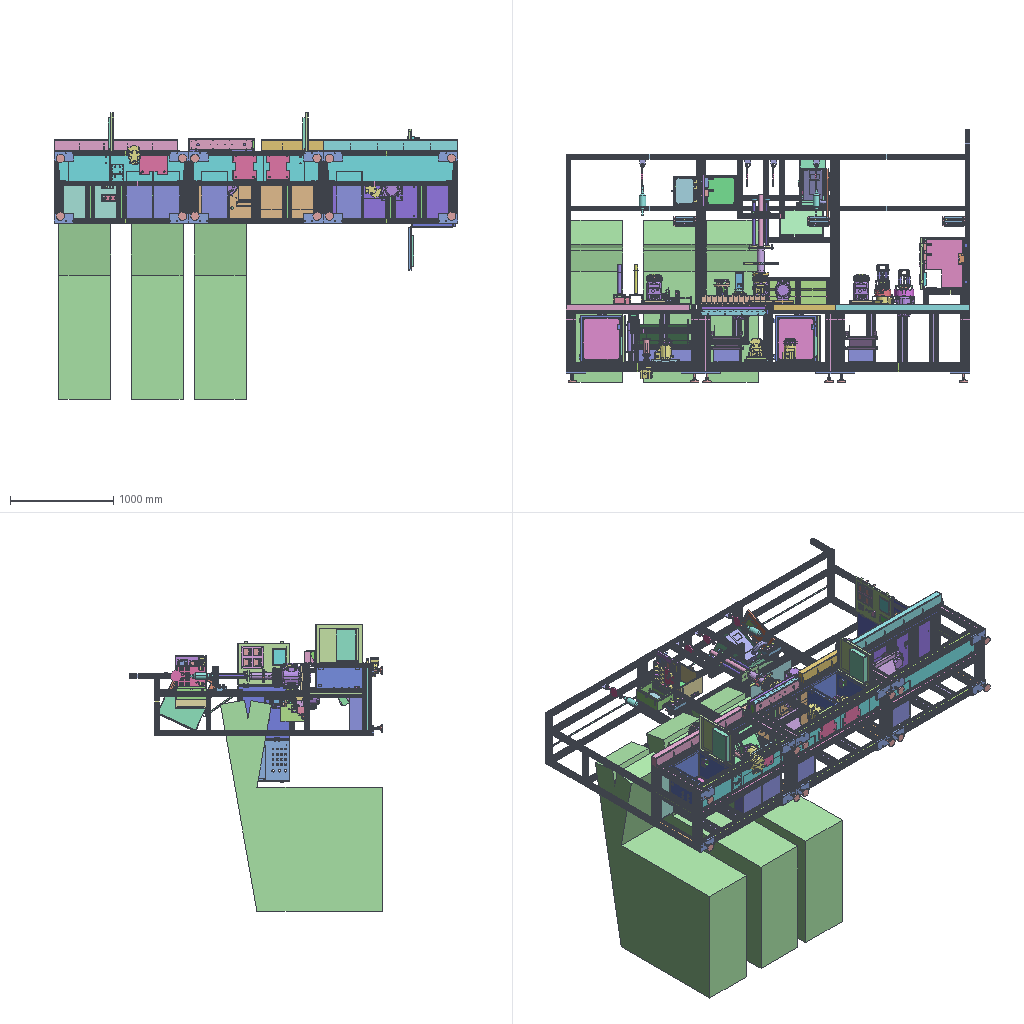Assembly | STEP file | 253 different items | 762 placed | box 3900 x 2440 x 2771 mm
Parts list (item | name | quantity | parent item | size | volume):
1 | Foot pad | x12 | in 1300 standard stand 3 | 80 x 145 x 80 mm | 114495 mm3
2 | Foot seat plate 2 | x12 | in 1300 standard stand 3 | 190 x 100 x 20 mm | 368452 mm3
3 | 4590-1120 aluminium profile (bottom rear cross 2) | x6 | in 1300 standard stand 3 | 90 x 45 x 1120 mm | 1313429 mm3
4 | 4590-705 Al 3 (front col) | x6 | in 1300 standard stand 3 | 90 x 45 x 558 mm | 654369 mm3
5 | 4590-600 Al (base long) | x6 | in 1300 standard stand 3 | 90 x 45 x 610 mm | 715349 mm3
6 | 4590-705 aluminium profile (rear column 2) | x6 | in 1300 standard stand 3 | 90 x 45 x 603 mm | 707141 mm3
7 | 4590-615 aluminium profile (rear middle upright 2) | x9 | in 1300 standard stand 3 | 90 x 45 x 513 mm | 601597 mm3
8 | 4590 aluminium profile (middle longitudinal 3) | x15 | in 1300 standard stand 3 | 90 x 45 x 700 mm | 820893 mm3
9 | 4545-1210 aluminium profile (upper long) | x12 | in 1300 standard stand 3 | 45 x 45 x 1407 mm | 976243 mm3
10 | 4545-1210 aluminium profile (upper cross long) | x14 | in 1300 standard stand 3 | 45 x 45 x 1210 mm | 839555 mm3
11 | 4545-765 aluminium profile (upper short) | x6 | in 1300 standard stand 3 | 45 x 45 x 597.5 mm | 414574 mm3
12 | SOP hanger seat | x6 | in 1300 standard stand 3 | 50 x 30 x 28 mm | 13038 mm3
13 | SOP hanger | x3 | in 1300 standard stand 3 | 12 x 12 x 1210 mm | 136812 mm3
14 | 4545-390 Al (side support) | x6 | in 1300 standard stand 3 | 45 x 45 x 335 mm | 232439 mm3
15 | 4590-1300 | x3 | in 1300 standard stand 3 | 90 x 45 x 1300 mm | 1524515 mm3
16 | 4590 Al (column) | x6 | in 1300 standard stand 3 | 90 x 45 x 513 mm | 601597 mm3
17 | 4590-1210 aluminium profile | x3 | in 1300 standard stand 3 | 90 x 45 x 1210 mm | 1418972 mm3
18 | Jig plate | x3 | in 1300 standard stand 3 | 1300 x 337.75 x 2 mm | 788863 mm3
19 | 10P30 assy jig base | x3 | in 10P30 assy locating jig | 230 x 270 x 25 mm | 1350745 mm3
20 | PN_0001 cylinder body | x7 | in 10P30 | 246.9 x 192 x 142 mm | 3389900 mm3
21 | PN_0001 rotor | x8 | in 10P30, Rotor mis-part check fixture | 43.5 x 155 x 155 mm | 349048 mm3
22 | 10P30 rotor 2 | x8 | in 10P30, Rotor mis-part check fixture | 43.5 x 156.4 x 156.4 mm | 346928 mm3
23 | 10P30 rotor clip | x8 | in 10P30, Circlip fixture (PN_0001 rotor) | 48.3 x 51.304 x 1.75 mm | 1045 mm3
24 | 10P30 hub | x8 | in 10P30, Shim selector hub step measuring fixture | 45 x 134.5 x 134.5 mm | 158986 mm3
25 | 10P30 stator | x7 | in 10P30 | 133.205 x 156.603 x 50 mm | 289241 mm3
26 | prevailing torque hex nuts with flange gb_PreviewCfg | x7 | in 10P30 | 11.8 x 11.8 x 5.3 mm | 298.912 mm3
27 | Fixture base plate | x6 | in 10P30 assy locating jig, Mkt assy locating jig | 270 x 230 x 15 mm | 846944 mm3
28 | Market locating fixture base plate | x3 | in Mkt assy locating jig | 230 x 270 x 25 mm | 1234801 mm3
29 | Market cylinder body | x7 | in Market, Stator circlip shortage check fixture | 195.5 x 183.011 x 125.785 mm | 2010849 mm3
30 | Market rotor | x7 | in Market, Rotor mis-part check fixture | 30.5 x 135 x 135 mm | 165270 mm3
31 | Mkt rotor clip | x7 | in Market, Circlip fixture (market rotor) | 41.6 x 41.383 x 1 mm | 557.011 mm3
32 | Market stator | x6 | in Market | 29.5 x 96.5 x 96.5 mm | 131288 mm3
33 | Mkt stator clip | x9 | in Market, Stator circlip shortage check fixture, Circlip fixture (market stator) | 43.8 x 47.287 x 1.8 mm | 874.267 mm3
34 | Mkt hub | x7 | in Market, Shim selector hub step measuring fixture | 38 x 105 x 105 mm | 81740 mm3
35 | hexagon flange bolts--small series gb_PreviewCfg | x6 | in Market | 31.8 x 13.6 x 13.6 mm | 1212 mm3
36 | Outer collar ring | x1 | in Stator circlip shortage check fixture | 72 x 72 x 57 mm | 42154 mm3
37 | Inner collar ring | x1 | in Stator circlip shortage check fixture | 41 x 41 x 43 mm | 18386 mm3
38 | Sensing post | x1 | in Stator circlip shortage check fixture | 11 x 15 x 29 mm | 1328 mm3
39 | Sensor mounting seat | x1 | in Stator circlip shortage check fixture | 72 x 72 x 46.3 mm | 26633 mm3
40 | Fix sleeve | x1 | in Stator circlip shortage check fixture | 72 x 72 x 150.6 mm | 87626 mm3
41 | Sensor nut | x1 | in Stator circlip shortage check fixture | 13 x 13.856 x 16.3 mm | 789.56 mm3
42 | Sensor head GT2-H12 | x1 | in Stator circlip shortage check fixture | 28 x 118.4 x 16 mm | 29940 mm3
43 | Return spring | x1 | in Stator circlip shortage check fixture | 32.75 x 32.75 x 12.75 mm | 176.657 mm3
44 | Stator clip std part | x1 | in Stator circlip shortage check fixture | 22 x 70 x 70 mm | 50341 mm3
45 | Stator circlip gauge hook | x1 | in Stator circlip shortage check fixture | 70 x 102 x 6 mm | 7420 mm3
46 | Spring hanging buckle | x4 | in Spring scale hook | 70 x 82.5 x 5 mm | 17833 mm3
47 | Spring hanger hook | x4 | in Spring scale hook | 18 x 8 x 120 mm | 16287 mm3
48 | Spring scale | x4 | in Spring scale hook | 106.116 x 223.189 x 10 mm | 107592 mm3
49 | Base-10P30 rotor clip | x1 | in Circlip fixture (PN_0001 rotor) | 120 x 86 x 10 mm | 99024 mm3
50 | Circlip fixture-upright plate | x8 | in Circlip fixture (PN_0001 rotor), Circlip fixture (market stator), Circlip fixture (market rotor) | 86 x 80 x 10 mm | 66708 mm3
51 | Clip jig-top plate | x4 | in Circlip fixture (PN_0001 rotor), Circlip fixture (market stator), Circlip fixture (market rotor) | 120 x 76 x 10 mm | 73644 mm3
52 | Clip jig-column 1 | x4 | in Circlip fixture (PN_0001 rotor), Circlip fixture (market stator), Circlip fixture (market rotor) | 15 x 12 x 291 mm | 49759 mm3
53 | Conn plate L | x3 | in Circlip fixture (PN_0001 rotor), Circlip fixture (market stator) | 40 x 288.5 x 1 mm | 11349 mm3
54 | Circlip fixture-medium storage post | x1 | in Circlip fixture (PN_0001 rotor) | 39 x 38.994 x 288.5 mm | 253295 mm3
55 | Strip (L) | x3 | in Circlip fixture (PN_0001 rotor), Circlip fixture (market stator) | 15 x 2 x 288.5 mm | 8464 mm3
56 | Photo seat | x8 | in Circlip fixture (PN_0001 rotor), Circlip fixture (market stator), Circlip fixture (market rotor) | 35 x 20 x 2 mm | 1235 mm3
57 | Circlip fixture-column 2 | x4 | in Circlip fixture (PN_0001 rotor), Circlip fixture (market stator), Circlip fixture (market rotor) | 15 x 12 x 291 mm | 51262 mm3
58 | Base plate-market stator circlip | x2 | in Circlip fixture (market stator) | 120 x 86 x 10 mm | 98205 mm3
59 | Circlip fixture-large storage post | x2 | in Circlip fixture (market stator) | 35.5 x 35.493 x 288.5 mm | 209417 mm3
60 | Base plate-market rotor circlip | x1 | in Circlip fixture (market rotor) | 120 x 86 x 10 mm | 97902 mm3
61 | Press strip (small) | x1 | in Circlip fixture (market rotor) | 12 x 2 x 289.5 mm | 6757 mm3
62 | Conn plate (S) | x1 | in Circlip fixture (market rotor) | 35 x 289.5 x 1 mm | 9942 mm3
63 | Clip jig-small post | x1 | in Circlip fixture (market rotor) | 30 x 29.992 x 289.3 mm | 149299 mm3
64 | Rotor mismatch side plate | x2 | in Rotor mis-part check fixture | 200 x 65 x 12 mm | 150424 mm3
65 | Rotor mis-part check fixture-guide rod | x4 | in Rotor mis-part check fixture | 12 x 12 x 210 mm | 23681 mm3
66 | Rotor mis-part check fixture-base plate | x1 | in Rotor mis-part check fixture | 440 x 200 x 11 mm | 944706 mm3
67 | Rotor mismatch mid plate | x2 | in Rotor mis-part check fixture | 200 x 54 x 12 mm | 123822 mm3
68 | Rotor mis-part check fixture-go gauge 1 | x1 | in Rotor mis-part check fixture | 200 x 120 x 12 mm | 206238 mm3
69 | Rotor mismatch gauge 2 | x1 | in Rotor mis-part check fixture | 200 x 120 x 12 mm | 185907 mm3
70 | Rotor mismatch gauge 3 | x1 | in Rotor mis-part check fixture | 200 x 120 x 12 mm | 185482 mm3
71 | Rotor detection photoelectric sensor | x2 | in Rotor mis-part check fixture | 29.674 x 4 x 54.352 mm | 340.68 mm3
72 | Rotor photoelectric sensor bracket | x1 | in Rotor mis-part check fixture | 80 x 106 x 15 mm | 26188 mm3
73 | Proximity mount-rotor | x2 | in Rotor mis-part check fixture | 66 x 40 x 20 mm | 4954 mm3
74 | Knob plunger PMXYK10 | x2 | in Rotor mis-part check fixture | 18 x 52 x 18 mm | 5094 mm3
75 | Guide rod connection | x2 | in Rotor mis-part check fixture | 12 x 11 x 16 mm | 1579 mm3
76 | hexagon socket head cap screws gb_PreviewCfg | x6 | in Rotor mis-part check fixture, 35N wrench lock | 7.6 x 3 x 3 mm | 21.652 mm3
77 | Shim select base | x1 | in Shim selector hub step measuring fixture | 150 x 150 x 12 mm | 250622 mm3
78 | Column | x3 | in Shim selector hub step measuring fixture | 16 x 16 x 160 mm | 30717 mm3
79 | Shim selection fixture body | x1 | in Shim selector hub step measuring fixture | 150 x 150 x 50 mm | 396055 mm3
80 | GS-1713 (Ono) | x11 | in Shim selector hub step measuring fixture, Rotor step measuring fixture-PN_0001, Clearance measuring fixture-PN_0001, Gap jig-Mkt | 18 x 33 x 141.5 mm | 52927 mm3
81 | GS mount plate | x1 | in Shim selector hub step measuring fixture | 50 x 75 x 8 mm | 29332 mm3
82 | Guide post | x1 | in Shim selector hub step measuring fixture | 10 x 12 x 44 mm | 1435 mm3
83 | Spring-hub step test | x1 | in Shim selector hub step measuring fixture | 8.7 x 8.7 x 23.95 mm | 74.991 mm3
84 | Guide post cap | x1 | in Shim selector hub step measuring fixture | 11.5 x 11.5 x 8 mm | 657.251 mm3
85 | PN_0001 hub standard part | x1 | in Shim selector hub step measuring fixture | 134.5 x 134.5 x 16.35 mm | 127475 mm3
86 | Mkt hub std part | x1 | in Shim selector hub step measuring fixture | 105 x 105 x 11.7 mm | 77844 mm3
87 | Prox bracket-hub | x1 | in Shim selector hub step measuring fixture | 56 x 10 x 18 mm | 1998 mm3
88 | Probe guide bush JBA6-16 | x1 | in Shim selector hub step measuring fixture | 10 x 10 x 16 mm | 793.757 mm3
89 | Limit sleeve | x1 | in Shim selector hub step measuring fixture | 18.5 x 20 x 42.5 mm | 8069 mm3
90 | Sensor fixing block-10P30 | x1 | in Rotor step measuring fixture-PN_0001 | 70 x 80 x 57 mm | 133616 mm3
91 | Rotor locating claw-PN_0001 | x1 | in Rotor step measuring fixture-PN_0001 | 91.977 x 95 x 57 mm | 127328 mm3
92 | Small circlip installation check head-PN_0001 | x1 | in Rotor step measuring fixture-PN_0001 | 70 x 70 x 15.85 mm | 18313 mm3
93 | Circlip check locating post-PN_0001 | x3 | in Rotor step measuring fixture-PN_0001 | 15 x 15 x 52.5 mm | 2401 mm3
94 | Sensor mount plate | x10 | in Rotor step measuring fixture-PN_0001, Clearance measuring fixture-PN_0001, Gap jig-Mkt | 15 x 15 x 26 mm | 1338 mm3
95 | Rotor step probe-10P30 | x1 | in Rotor step measuring fixture-PN_0001 | 25 x 25 x 61.5 mm | 22119 mm3
96 | Rotor step cover | x1 | in Rotor step measuring fixture-PN_0001 | 85 x 75 x 160 mm | 109085 mm3
97 | Spring-circlip check | x1 | in Rotor step measuring fixture-PN_0001 | 41.5 x 41.5 x 26.5 mm | 1389 mm3
98 | Spring-rotor test | x1 | in Rotor step measuring fixture-PN_0001 | 18.75 x 18.75 x 28.75 mm | 175.083 mm3
99 | Rotor step bushing JBH8-12 | x3 | in Rotor step measuring fixture-PN_0001 | 16 x 16 x 16 mm | 1313 mm3
100 | hex nuts, style 1-grades ab gb_PreviewCfg | x3 | in Rotor step measuring fixture-PN_0001 | 18.475 x 16 x 8.4 mm | 1302 mm3
101 | Seat bracket-10P30 | x1 | in Rotor step measuring fixture-PN_0001 | 150 x 120 x 50 mm | 90314 mm3
102 | Seat-PN_0001 | x1 | in Rotor step measuring fixture-PN_0001 | 105 x 105 x 30 mm | 196684 mm3
103 | 35N torque tester | x1 | in 35N wrench lock | 54 x 85 x 717 mm | 972742 mm3
104 | Hex head-Mkt | x1 | in 35N wrench lock | 21 x 21 x 80 mm | 24655 mm3
105 | Hub mounting plate | x1 | in 35N wrench lock | 155 x 155 x 30 mm | 252907 mm3
106 | Connecting tube sleeve | x1 | in 35N wrench lock | 70 x 70 x 230 mm | 273867 mm3
107 | Bush plate | x1 | in 35N wrench lock | 180 x 180 x 15 mm | 370713 mm3
108 | Handle seat new 2 | x1 | in 35N wrench lock | 68.5 x 120 x 20 mm | 86648 mm3
109 | Handle seat new 1 | x1 | in 35N wrench lock | 68.5 x 120 x 20 mm | 85047 mm3
110 | Handle new | x2 | in 35N wrench lock | 20 x 20 x 112 mm | 31180 mm3
111 | A2A-4B | x1 | in 35N wrench lock | 20 x 41.8 x 14 mm | 7935 mm3
112 | Wrench hook | x2 | in 35N wrench lock | 26 x 26 x 6 mm | 1260 mm3
113 | Linear bearing LMH25UU | x2 | in 35N wrench lock | 59 x 62 x 46 mm | 53686 mm3
114 | 25 guide rod | x2 | in 35N wrench lock | 25 x 25 x 450 mm | 219459 mm3
115 | Wrench mounting plate | x1 | in 35N wrench lock | 240 x 100 x 15 mm | 319377 mm3
116 | 4545 profile 1 | x2 | in 35N wrench lock | 45 x 45 x 450 mm | 312231 mm3
117 | Hard stop block | x2 | in 35N wrench lock | 50 x 50 x 20 mm | 36960 mm3
118 | Buffer sleeve | x2 | in 35N wrench lock | 50 x 50 x 20 mm | 26853 mm3
119 | 4545 profile 2 | x2 | in 35N wrench lock | 45 x 45 x 535 mm | 371208 mm3
120 | 4545 profile 3 | x2 | in 35N wrench lock | 45 x 45 x 90 mm | 62446 mm3
121 | Hub chuck-Mkt | x1 | in 35N wrench lock | 135 x 135 x 18 mm | 146789 mm3
122 | Hex head-PN_0001 | x1 | in 35N wrench lock | 21 x 21 x 90 mm | 27340 mm3
123 | Hub chuck-10P | x1 | in 35N wrench lock | 135 x 135 x 18 mm | 101128 mm3
124 | Torsion pin | x2 | in 35N wrench lock | 10 x 10 x 20 mm | 1542 mm3
125 | Torque wrench | x2 | - | 63.096 x 292.35 x 63.096 mm | 430044 mm3
126 | Screw lock-base plate PN_0001 | x1 | in Screw lock jig 10P30 | 270 x 200 x 25 mm | 1267432 mm3
127 | Screw jig plate | x2 | in Screw lock jig 10P30, Screw lock locating fixture-market | 200 x 270 x 15 mm | 725684 mm3
128 | Flange-10P30 | x1 | in Clearance measuring fixture-PN_0001 | 168 x 168 x 42 mm | 255273 mm3
129 | Conductive post-PN_0001 | x1 | in Clearance measuring fixture-PN_0001 | 11 x 11 x 94 mm | 4420 mm3
130 | Handle rod | x2 | in Clearance measuring fixture-PN_0001, Gap jig-Mkt | 32 x 32 x 94 mm | 15016 mm3
131 | Handle seat | x2 | in Clearance measuring fixture-PN_0001, Gap jig-Mkt | 137 x 24.5 x 15 mm | 45015 mm3
132 | Gap jig seat-10P30 | x1 | in Clearance measuring fixture-PN_0001 | 190 x 190 x 65 mm | 588080 mm3
133 | Fixture seat bracket-PN_0001 | x1 | in Clearance measuring fixture-PN_0001 | 200 x 200 x 80 mm | 215628 mm3
134 | Locating post-10P30 | x1 | in Clearance measuring fixture-PN_0001 | 65 x 65 x 33 mm | 42831 mm3
135 | Handle | x2 | in Clearance measuring fixture-PN_0001, Gap jig-Mkt | 137 x 42 x 26 mm | 58032 mm3
136 | Spring | x2 | in Clearance measuring fixture-PN_0001, Gap jig-Mkt | 10.75 x 10.75 x 22 mm | 58.932 mm3
137 | Proximity mounting bent plate | x2 | in Clearance measuring fixture-PN_0001, Gap jig-Mkt | 30 x 32 x 45 mm | 1657 mm3
138 | Guard post | x8 | in Clearance measuring fixture-PN_0001, Gap jig-Mkt | 10 x 10 x 45 mm | 3034 mm3
139 | Station two ctrl box body | x1 | in Station two ctrl box | 310 x 300 x 225.796 mm | 688947 mm3
140 | Station two ctrl box cover | x1 | in Station two ctrl box | 300 x 20 x 300 mm | 151242 mm3
141 | Station two mount plate | x1 | in Station two ctrl box | 270 x 270 x 17 mm | 174541 mm3
142 | Amplifier | x6 | in Station two ctrl box, Station three ctrl box | 72 x 72 x 119 mm | 337581 mm3
143 | Shim selection | x1 | in Station two ctrl box | 96 x 96 x 119 mm | 593520 mm3
144 | Button | x10 | in Station two ctrl box, Station three ctrl box | 24 x 20 x 39 mm | 10735 mm3
145 | Display 1 | x2 | in Station two ctrl box, Station three ctrl box | 68 x 33 x 10 mm | 22440 mm3
146 | Selector switch | x1 | in Station two ctrl box | 25 x 25 x 30 mm | 7576 mm3
147 | DIP switch | x3 | in Station two ctrl box | 40 x 30 x 5.5 mm | 6025 mm3
148 | Hinge leaf | x8 | in Station two ctrl box, Station three ctrl box | 25.5 x 24.5 x 54 mm | 7881 mm3
149 | Hinge shaft | x6 | in Station two ctrl box, Station three ctrl box | 6 x 54 x 6 mm | 1527 mm3
150 | Station two plug plate low | x2 | in Station two ctrl box | 85 x 10 x 17.5 mm | 12524 mm3
151 | Station two plug plate up | x2 | in Station two ctrl box | 85 x 10 x 17.5 mm | 11964 mm3
152 | DIP switch expansion board | x1 | in Station two ctrl box | 285 x 75 x 8 mm | 128331 mm3
153 | Ctrl box POM plate | x8 | in Station two ctrl box, Upper control box.SLDPRT1, Lower electrical control box 1 | 100 x 5 x 22.5 mm | 9009 mm3
154 | Station three ctrl box body | x1 | in Station three ctrl box | 420 x 500 x 524 mm | 2167031 mm3
155 | Station three ctrl box cover | x1 | in Station three ctrl box | 500 x 24 x 420 mm | 428916 mm3
156 | Station three mount plate | x2 | in Station three ctrl box | 460 x 376 x 2 mm | 291324 mm3
157 | Touch screen | x1 | in Station three ctrl box | 165 x 135 x 59.8 mm | 1170552 mm3
158 | Buzzer | x1 | in Station three ctrl box | 16.5 x 16.5 x 5 mm | 1069 mm3
159 | Buzzer large | x1 | in Station three ctrl box | 22.5 x 22.5 x 5 mm | 1988 mm3
160 | Display 2 | x1 | in Station three ctrl box | 72 x 100 x 10 mm | 72000 mm3
161 | Mirror hinge leaf | x4 | in Station three ctrl box | 25.5 x 24.5 x 54 mm | 7881 mm3
162 | Station three ctrl box rear cover | x1 | in Station three ctrl box | 500 x 24 x 410 mm | 510140 mm3
163 | Acrylic cover plate | x1 | in Station three ctrl box | 80 x 120 x 5 mm | 47734 mm3
164 | Acrylic cover 2 | x1 | in Station three ctrl box | 210 x 210 x 5 mm | 220075 mm3
165 | Manual box | x3 | in Station three ctrl box, Lower electrical control box 1 | 334 x 192 x 50 mm | 192178 mm3
166 | Three-control-box air switch | x1 | in Station three ctrl box | 100 x 84.014 x 49.5 mm | 273026 mm3
167 | Three-control-box air switch baffle | x1 | in Station three ctrl box | 154 x 50 x 60 mm | 23219 mm3
168 | Upper control box 1 | x1 | in Upper control box.SLDPRT1 | 241 x 290 x 131.995 mm | 409280 mm3
169 | Upper control box cover | x1 | in Upper control box.SLDPRT1 | 224 x 290 x 22 mm | 182684 mm3
170 | Ctrl board 11 | x1 | in Upper control box.SLDPRT1 | 175 x 245 x 10 mm | 97407 mm3
171 | Start button AR22EOL-10E3G_Fuji1_default | x9 | in Upper control box.SLDPRT1 | 77.5 x 42 x 30 mm | 58541 mm3
172 | Start button AR22EOL-10E3G11_Fuji1_default | x1 | in Upper control box.SLDPRT1 | 77.5 x 42 x 30 mm | 58541 mm3
173 | Hinge leaf 11 | x16 | in Upper control box.SLDPRT1, Lower electrical control box 1, Hinge 1 | 25.5 x 24.5 x 54 mm | 7881 mm3
174 | Hinge shaft 11 | x8 | in Upper control box.SLDPRT1, Lower electrical control box 1, Hinge 1 | 6 x 54 x 6 mm | 1527 mm3
175 | Lower ctrl box 1 | x2 | in Lower electrical control box 1 | 415 x 450 x 322.745 mm | 1529445 mm3
176 | Lower ctrl cover 1 | x2 | in Lower electrical control box 1 | 400 x 450 x 26 mm | 580163 mm3
177 | Lower control board 11 | x2 | in Lower electrical control box 1 | 350 x 400 x 12 mm | 307444 mm3
178 | Power switch 1 | x2 | in Lower electrical control box 1 | 55 x 49.883 x 40.112 mm | 61552 mm3
179 | Socket 1 | x2 | in Lower electrical control box 1 | 50 x 100 x 10 mm | 43682 mm3
180 | Air switch plate 1 | x2 | in Lower electrical control box 1 | 79 x 45 x 2 mm | 6983 mm3
181 | Air switch blank | x2 | in Lower electrical control box 1 | 80 x 44 x 49 mm | 14511 mm3
182 | Indicator plate | x3 | in 185 | 220 x 88.473 x 10.009 mm | 42803 mm3
183 | Indicator light board | x3 | in 185 | 184 x 94 x 50 mm | 80341 mm3
184 | Indicator light red | x15 | in 185 | 25 x 20 x 37 mm | 13712 mm3
185 | Indicator | x15 | in 185 | 25 x 20 x 37 mm | 13712 mm3
186 | Cabinet body | x1 | in Wrench controller box cabinet | 310 x 447.968 x 304.324 mm | 1012965 mm3
187 | Cabinet cover | x1 | in Wrench controller box cabinet | 246 x 406 x 22 mm | 265621 mm3
188 | Wrench controller | x1 | in Wrench controller box cabinet | 295.575 x 373.272 x 365 mm | 11651636 mm3
189 | Wrench controller display guard | x1 | in Wrench controller box cabinet | 156 x 126 x 5 mm | 97780 mm3
190 | Wrench controller box rear cover | x1 | in Wrench controller box cabinet | 246 x 406 x 17 mm | 220004 mm3
191 | PC rack top (asm 3) | x1 | in PC rack | 650 x 448 x 2.5 mm | 688011 mm3
192 | 4545-650 Al (PC rack 1) | x2 | in PC rack | 45 x 45 x 650 mm | 451001 mm3
193 | 4545-400 aluminium profile (computer rack assembly 2) | x2 | in PC rack | 45 x 45 x 358 mm | 248397 mm3
194 | Computer | x1 | in PC rack | 420 x 320 x 238.828 mm | 1582397 mm3
195 | 4545 Al PC rack upright | x1 | in PC rack | 45 x 45 x 758.77 mm | 526470 mm3
196 | 4545 aluminium computer rack upper cross | x1 | in PC rack | 45 x 45 x 172.5 mm | 119689 mm3
197 | 4545-400 Al (rack asm 1) | x2 | in Station three ctrl box rack | 45 x 45 x 400 mm | 277539 mm3
198 | 4545-330 Al (rack asm 2) | x2 | in Station three ctrl box rack | 45 x 45 x 335 mm | 232439 mm3
199 | 4545-100 Al (rack asm 3) | x4 | in Station three ctrl box rack | 45 x 45 x 100 mm | 69385 mm3
200 | Seal sleeve 1 | x1 | in 226 | 18 x 18 x 43 mm | 8232 mm3
201 | Guard plate | x1 | in 226 | 170 x 50 x 8 mm | 48727 mm3
202 | Seal sleeve 2 | x1 | in 226 | 19.5 x 18 x 43 mm | 8218 mm3
203 | Seal sleeve 5 | x1 | in 226 | 20 x 20 x 43 mm | 8055 mm3
204 | Seal sleeve 6 | x1 | in 226 | 20 x 21.865 x 43 mm | 7995 mm3
205 | Seal sleeve 7 | x1 | in 226 | 25 x 21.651 x 43 mm | 9390 mm3
206 | Seal sleeve 8 | x1 | in 226 | 26 x 19.919 x 43 mm | 9352 mm3
207 | hex socket set screws with flat point gb_PreviewCfg | x1 | in 226 | 3 x 1.6 x 1.6 mm | 5.35 mm3
208 | Seal lower box | x1 | in 226 | 170 x 50 x 22 mm | 92795 mm3
209 | Proximity m8 | x1 | in 226 | 8 x 8 x 30 mm | 1210 mm3
210 | Printer | x2 | in Nameplate holder | 260 x 230 x 250 mm | 14489193 mm3
211 | Light curtain | x6 | in Nameplate holder, Seal pick-and-place box | 144 x 34 x 10 mm | 48175 mm3
212 | 3030 printer curtain rod | x3 | in Nameplate holder | 29.915 x 30.09 x 235 mm | 73681 mm3
213 | 3030 printer light curtain mount | x1 | in Nameplate holder | 29.915 x 30.09 x 629.59 mm | 197400 mm3
214 | Storage box shell | x1 | in Shim storage box split 1 | 122 x 53 x 633 mm | 271633 mm3
215 | Storage display board | x1 | in Shim storage box split 1 | 30 x 33 x 626 mm | 79983 mm3
216 | Storage insert | x1 | in Shim storage box split 1 | 86 x 45 x 626 mm | 245916 mm3
217 | Chrome small handle | x12 | in Shim storage box split 1 | - | 5297 mm3
218 | Hinge shaft 1 | x1 | in Shim storage box split 1 | 2 x 30 x 2 mm | 94.248 mm3
219 | Hinge leaf 1 | x24 | in Shim storage box split 1 | 15.5 x 3.5 x 30 mm | 454.79 mm3
220 | Storage prox plate | x1 | in Shim storage box split 1 | 17 x 43 x 626 mm | 73636 mm3
221 | Box cover | x12 | in Shim storage box split 1 | 92.738 x 7.788 x 51 mm | 9373 mm3
222 | Shim lower mounting plate 2 | x1 | in Shim storage box split 1 | 633 x 50 x 12 mm | 367777 mm3
223 | Shim front mounting plate | x2 | in Shim storage box split 1 | 98 x 50 x 12 mm | 58113 mm3
224 | Shim mounting plate base | x1 | in Shim storage box split 1 | 607 x 98 x 12 mm | 699324 mm3
225 | Shim lower plate | x1 | in Shim storage box split 1 | 633 x 50 x 12 mm | 358808 mm3
226 | Seal box | x1 | in Seal pick-and-place box | 137.473 x 200 x 60 mm | 159920 mm3
227 | NG chute L | x2 | - | 400 x 320 x 147.024 mm | 579162 mm3
228 | NG chute S | x2 | - | 450 x 268 x 103.148 mm | 495512 mm3
229 | 3030-200 | x3 | - | 29.915 x 30.09 x 220 mm | 68984 mm3
230 | 4545-240 Al (tri-LED mount) | x1 | - | 45 x 45 x 240 mm | 166523 mm3
231 | Screw lock-base Mkt | x1 | in Screw lock locating fixture-market | 270 x 200 x 25 mm | 1265515 mm3
232 | Screw lock-middle support | x1 | in Screw lock locating fixture-market | 160 x 40 x 22 mm | 96700 mm3
233 | 1300 table 1 | x1 | - | 1300 x 700 x 2 mm | 1751949 mm3
234 | 1300 table top 2 | x1 | - | 1300 x 700 x 2 mm | 1762203 mm3
235 | 1300 table top 3 | x1 | - | 1300 x 700 x 2 mm | 1765463 mm3
236 | Material rack | x3 | - | 500 x 1564 x 2041 mm | 933674835 mm3
237 | Clip connector box | x1 | in 237 | 174 x 70 x 70 mm | 79761 mm3
238 | Aviation connector M16-8AB | x3 | in 237 | 16.5 x 24 x 20.785 mm | 3887 mm3
239 | Jig prox plate | x8 | - | 51 x 15 x 11 mm | 1646 mm3
240 | 4545 profile NG mount | x2 | - | 45 x 45 x 585 mm | 405901 mm3
241 | 4545 profile NG mount 2 | x1 | - | 45 x 45 x 143 mm | 99220 mm3
242 | 4545 profile NG mount 3 | x1 | - | 45 x 45 x 375 mm | 260193 mm3
243 | NG parts material box | x4 | - | 450 x 250 x 120 mm | 553512 mm3
244 | 4545-250 | x1 | - | 45 x 45 x 250 mm | 173462 mm3
245 | Sheet metal material box large | x1 | - | 1190 x 110 x 92 mm | 652065 mm3
246 | Sheet box 1300 | x1 | - | 1300 x 110 x 92 mm | 708554 mm3
247 | Sheet metal material box | x1 | - | 595 x 110 x 92 mm | 340939 mm3
248 | Flange-market | x1 | in Gap jig-Mkt | 138 x 138 x 40 mm | 168413 mm3
249 | Conductive post-market | x1 | in Gap jig-Mkt | 11 x 11 x 83 mm | 4143 mm3
250 | Clearance measuring fixture seat-market | x1 | in Gap jig-Mkt | 155 x 155 x 65 mm | 392527 mm3
251 | Fixture seat bracket-market | x1 | in Gap jig-Mkt | 200 x 180 x 80 mm | 194275 mm3
252 | Locating post-Mkt | x1 | in Gap jig-Mkt | 55 x 55 x 33 mm | 35166 mm3
253 | Anti-rot sleeve | x1 | in Gap jig-Mkt | 9 x 9 x 6 mm | 238.468 mm3
Placements (level | parent | child | x y z in mm | rotation matrix by rows), first 254 of 819 lines:
1 | subassembly 2 | 1300 standard stand 3 | -1605.684 -1063.748 235.0 | 1 0 0 0 1 0 0 0 1
2 | 1300 standard stand 3 | Foot pad | -24.63 -37.019 -0.0 | 1 0 0 0 1 0 0 0 1
2 | 1300 standard stand 3 | Foot seat plate 2 | -84.63 42.981 -30.0 | 1 0 0 0 0 1 0 -1 0
2 | 1300 standard stand 3 | 4590-1120 aluminium profile (bottom rear cross 2) | 1125.37 3826.208 -7183.709 | 0 0 -1 -1 0 0 0 1 0
2 | 1300 standard stand 3 | 4590-705 Al 3 (front col) | -3757.856 620.981 -7183.709 | 1 0 0 0 0 -1 0 1 -0
2 | 1300 standard stand 3 | 4590-600 Al (base long) | -7293.339 3826.208 -585.0 | 0 1 0 -1 0 0 0 0 1
2 | 1300 standard stand 3 | Foot seat plate 2 | -84.63 62.981 -530.0 | 1 0 0 0 0 -1 0 1 -0
2 | 1300 standard stand 3 | 4590-705 aluminium profile (rear column 2) | -3757.856 62.981 6623.709 | 1 0 0 0 0 1 0 -1 0
2 | 1300 standard stand 3 | 4590-1120 aluminium profile (bottom rear cross 2) | 5.37 3826.208 6623.709 | 0 0 1 -1 0 0 0 -1 0
2 | 1300 standard stand 3 | 4590-705 Al 3 (front col) | -2547.856 620.981 -7183.709 | 1 0 0 0 0 -1 0 1 -0
2 | 1300 standard stand 3 | 4590-705 aluminium profile (rear column 2) | 4888.597 665.981 6623.709 | -1 0 0 0 0 -1 0 -1 -0
2 | 1300 standard stand 3 | 4590-600 Al (base long) | -6038.339 3826.208 -585.0 | 0 1 0 -1 0 0 0 0 1
2 | 1300 standard stand 3 | Foot seat plate 2 | 1215.37 42.981 -530.0 | -1 0 0 0 0 1 0 1 0
2 | 1300 standard stand 3 | Foot seat plate 2 | 1215.37 62.981 -30.0 | -1 0 0 0 0 -1 0 -1 -0
2 | 1300 standard stand 3 | Foot pad | 1155.37 -37.019 -560.0 | -0.2377 0 -0.9713 0 1 0 0.9713 0 -0.2377
2 | 1300 standard stand 3 | Foot pad | 1155.37 -37.019 -0.0 | -0.6627 0 0.7489 0 1 0 -0.7489 0 -0.6627
2 | 1300 standard stand 3 | Foot pad | -24.63 -37.019 -560.0 | -0.3516 0 0.9361 0 1 0 -0.9361 0 -0.3516
2 | 1300 standard stand 3 | 4590-615 aluminium profile (rear middle upright 2) | -3455.356 152.981 6623.709 | 1 0 0 0 0 1 0 -1 -0
2 | 1300 standard stand 3 | 4590 aluminium profile (middle longitudinal 3) | -3757.856 -6542.728 -630.0 | 1 0 0 0 1 0 0 0 1
2 | 1300 standard stand 3 | 4590 aluminium profile (middle longitudinal 3) | -3455.356 -6542.728 -630.0 | 1 0 0 0 1 0 0 0 1
2 | 1300 standard stand 3 | 4590 aluminium profile (middle longitudinal 3) | -2547.856 -6542.728 -630.0 | 1 0 0 0 1 0 0 0 1
2 | 1300 standard stand 3 | 4545-1210 aluminium profile (upper long) | -3676.177 710.981 6623.613 | 1 0 0 0 0 1 0 -1 0
2 | 1300 standard stand 3 | 4545-1210 aluminium profile (upper cross long) | 1170.37 -5090.632 -4221.547 | 0 0 -1 0 1 0 1 0 -0
2 | 1300 standard stand 3 | 4545-1210 aluminium profile (upper long) | -3676.177 2117.981 -7458.613 | 1 0 0 0 0 -1 0 1 -0
2 | 1300 standard stand 3 | 4545-1210 aluminium profile (upper long) | -2421.177 2117.981 -7458.613 | 1 0 0 0 0 -1 0 1 -0
2 | 1300 standard stand 3 | 4545-1210 aluminium profile (upper cross long) | -39.63 -5090.632 3341.547 | 0 0 1 0 1 0 -1 0 -0
2 | 1300 standard stand 3 | 4545-1210 aluminium profile (upper cross long) | 1170.37 -5090.632 -3669.047 | 0 0 -1 0 1 0 1 0 0
2 | 1300 standard stand 3 | 4545-1210 aluminium profile (upper long) | -2421.177 710.981 6623.613 | 1 0 0 0 0 1 0 -1 0
2 | 1300 standard stand 3 | 4545-765 aluminium profile (upper short) | -2421.177 -5090.632 -630.0 | 1 0 0 0 1 0 0 0 1
2 | 1300 standard stand 3 | 4545-765 aluminium profile (upper short) | -3676.177 -5090.632 -630.0 | 1 0 0 0 1 0 0 0 1
2 | 1300 standard stand 3 | SOP hanger seat | 1170.37 2140.481 -445.0 | 0 0 -1 0 1 0 1 0 0
2 | 1300 standard stand 3 | SOP hanger seat | -39.63 2140.481 -445.0 | 0 0 1 0 1 0 -1 0 -0
2 | 1300 standard stand 3 | SOP hanger | 1186.805 2140.481 -445.0 | 0 0 -1 1 0 0 0 -1 0
2 | 1300 standard stand 3 | 4545-1210 aluminium profile (upper cross long) | 1170.37 -5590.632 -4221.547 | 0 0 -1 0 1 0 1 0 -0
2 | 1300 standard stand 3 | 4545-390 Al (side support) | -3676.177 -5590.632 -585.0 | 1 0 0 0 1 0 0 0 1
2 | 1300 standard stand 3 | 4545-390 Al (side support) | -2421.177 -5590.632 -585.0 | 1 0 0 0 1 0 0 0 1
2 | 1300 standard stand 3 | 4590-1300 | 565.37 -6587.728 -3693.227 | 0 0 -1 0 1 0 1 0 -0
2 | 1300 standard stand 3 | 4590 Al (column) | 8424.079 152.981 3495.477 | 0 -1 0 0 0 1 -1 0 0
2 | 1300 standard stand 3 | 4590 Al (column) | 7169.079 665.981 -3940.977 | 0 -1 0 0 0 -1 1 0 -0
2 | 1300 standard stand 3 | 4590-1210 aluminium profile | 1170.37 -3610.245 6985.959 | 0 0 -1 1 0 0 0 -1 0
2 | 1300 standard stand 3 | 4590 aluminium profile (middle longitudinal 3) | -3152.856 -6542.728 -630.0 | 1 0 0 0 1 0 0 0 1
2 | 1300 standard stand 3 | 4590-615 aluminium profile (rear middle upright 2) | -3152.856 152.981 6623.709 | 1 0 0 0 0 1 0 -1 -0
2 | 1300 standard stand 3 | 4590-615 aluminium profile (rear middle upright 2) | -2850.356 152.981 6623.709 | 1 0 0 0 0 1 0 -1 -0
2 | 1300 standard stand 3 | 4590 aluminium profile (middle longitudinal 3) | -2850.356 -6542.728 -630.0 | 1 0 0 0 1 0 0 0 1
2 | 1300 standard stand 3 | Jig plate | 565.37 152.981 -98.875 | 1 0 0 0 0 -1 0 1 -0
1 | subassembly 2 | 1300 standard stand 3 | -305.684 -1063.748 235.0 | 1 0 0 0 1 0 0 0 1
2 | 1300 standard stand 3 | Foot pad | -24.63 -37.019 -0.0 | 1 0 0 0 1 0 0 0 1
2 | 1300 standard stand 3 | Foot seat plate 2 | -84.63 42.981 -30.0 | 1 0 0 0 0 1 0 -1 0
2 | 1300 standard stand 3 | 4590-1120 aluminium profile (bottom rear cross 2) | 1125.37 3826.208 -7183.709 | 0 0 -1 -1 0 0 0 1 0
2 | 1300 standard stand 3 | 4590-705 Al 3 (front col) | -3757.856 620.981 -7183.709 | 1 0 0 0 0 -1 0 1 -0
2 | 1300 standard stand 3 | 4590-600 Al (base long) | -7293.339 3826.208 -585.0 | 0 1 0 -1 0 0 0 0 1
2 | 1300 standard stand 3 | Foot seat plate 2 | -84.63 62.981 -530.0 | 1 0 0 0 0 -1 0 1 -0
2 | 1300 standard stand 3 | 4590-705 aluminium profile (rear column 2) | -3757.856 62.981 6623.709 | 1 0 0 0 0 1 0 -1 0
2 | 1300 standard stand 3 | 4590-1120 aluminium profile (bottom rear cross 2) | 5.37 3826.208 6623.709 | 0 0 1 -1 0 0 0 -1 0
2 | 1300 standard stand 3 | 4590-705 Al 3 (front col) | -2547.856 620.981 -7183.709 | 1 0 0 0 0 -1 0 1 -0
2 | 1300 standard stand 3 | 4590-705 aluminium profile (rear column 2) | 4888.597 665.981 6623.709 | -1 0 0 0 0 -1 0 -1 -0
2 | 1300 standard stand 3 | 4590-600 Al (base long) | -6038.339 3826.208 -585.0 | 0 1 0 -1 0 0 0 0 1
2 | 1300 standard stand 3 | Foot seat plate 2 | 1215.37 42.981 -530.0 | -1 0 0 0 0 1 0 1 0
2 | 1300 standard stand 3 | Foot seat plate 2 | 1215.37 62.981 -30.0 | -1 0 0 0 0 -1 0 -1 -0
2 | 1300 standard stand 3 | Foot pad | 1155.37 -37.019 -560.0 | -0.2377 0 -0.9713 0 1 0 0.9713 0 -0.2377
2 | 1300 standard stand 3 | Foot pad | 1155.37 -37.019 -0.0 | -0.6627 0 0.7489 0 1 0 -0.7489 0 -0.6627
2 | 1300 standard stand 3 | Foot pad | -24.63 -37.019 -560.0 | -0.3516 0 0.9361 0 1 0 -0.9361 0 -0.3516
2 | 1300 standard stand 3 | 4590-615 aluminium profile (rear middle upright 2) | -3455.356 152.981 6623.709 | 1 0 0 0 0 1 0 -1 -0
2 | 1300 standard stand 3 | 4590 aluminium profile (middle longitudinal 3) | -3757.856 -6542.728 -630.0 | 1 0 0 0 1 0 0 0 1
2 | 1300 standard stand 3 | 4590 aluminium profile (middle longitudinal 3) | -3455.356 -6542.728 -630.0 | 1 0 0 0 1 0 0 0 1
2 | 1300 standard stand 3 | 4590 aluminium profile (middle longitudinal 3) | -2547.856 -6542.728 -630.0 | 1 0 0 0 1 0 0 0 1
2 | 1300 standard stand 3 | 4545-1210 aluminium profile (upper long) | -3676.177 710.981 6623.613 | 1 0 0 0 0 1 0 -1 0
2 | 1300 standard stand 3 | 4545-1210 aluminium profile (upper cross long) | 1170.37 -5090.632 -4221.547 | 0 0 -1 0 1 0 1 0 -0
2 | 1300 standard stand 3 | 4545-1210 aluminium profile (upper long) | -3676.177 2117.981 -7458.613 | 1 0 0 0 0 -1 0 1 -0
2 | 1300 standard stand 3 | 4545-1210 aluminium profile (upper long) | -2421.177 2117.981 -7458.613 | 1 0 0 0 0 -1 0 1 -0
2 | 1300 standard stand 3 | 4545-1210 aluminium profile (upper cross long) | -39.63 -5090.632 3341.547 | 0 0 1 0 1 0 -1 0 -0
2 | 1300 standard stand 3 | 4545-1210 aluminium profile (upper cross long) | 1170.37 -5090.632 -3669.047 | 0 0 -1 0 1 0 1 0 0
2 | 1300 standard stand 3 | 4545-1210 aluminium profile (upper long) | -2421.177 710.981 6623.613 | 1 0 0 0 0 1 0 -1 0
2 | 1300 standard stand 3 | 4545-765 aluminium profile (upper short) | -2421.177 -5090.632 -630.0 | 1 0 0 0 1 0 0 0 1
2 | 1300 standard stand 3 | 4545-765 aluminium profile (upper short) | -3676.177 -5090.632 -630.0 | 1 0 0 0 1 0 0 0 1
2 | 1300 standard stand 3 | SOP hanger seat | 1170.37 2140.481 -445.0 | 0 0 -1 0 1 0 1 0 0
2 | 1300 standard stand 3 | SOP hanger seat | -39.63 2140.481 -445.0 | 0 0 1 0 1 0 -1 0 -0
2 | 1300 standard stand 3 | SOP hanger | 1186.805 2140.481 -445.0 | 0 0 -1 1 0 0 0 -1 0
2 | 1300 standard stand 3 | 4545-1210 aluminium profile (upper cross long) | 1170.37 -5590.632 -4221.547 | 0 0 -1 0 1 0 1 0 -0
2 | 1300 standard stand 3 | 4545-390 Al (side support) | -3676.177 -5590.632 -585.0 | 1 0 0 0 1 0 0 0 1
2 | 1300 standard stand 3 | 4545-390 Al (side support) | -2421.177 -5590.632 -585.0 | 1 0 0 0 1 0 0 0 1
2 | 1300 standard stand 3 | 4590-1300 | 565.37 -6587.728 -3693.227 | 0 0 -1 0 1 0 1 0 -0
2 | 1300 standard stand 3 | 4590 Al (column) | 8424.079 152.981 3495.477 | 0 -1 0 0 0 1 -1 0 0
2 | 1300 standard stand 3 | 4590 Al (column) | 7169.079 665.981 -3940.977 | 0 -1 0 0 0 -1 1 0 -0
2 | 1300 standard stand 3 | 4590-1210 aluminium profile | 1170.37 -3610.245 6985.959 | 0 0 -1 1 0 0 0 -1 0
2 | 1300 standard stand 3 | 4590 aluminium profile (middle longitudinal 3) | -3152.856 -6542.728 -630.0 | 1 0 0 0 1 0 0 0 1
2 | 1300 standard stand 3 | 4590-615 aluminium profile (rear middle upright 2) | -3152.856 152.981 6623.709 | 1 0 0 0 0 1 0 -1 -0
2 | 1300 standard stand 3 | 4590-615 aluminium profile (rear middle upright 2) | -2850.356 152.981 6623.709 | 1 0 0 0 0 1 0 -1 -0
2 | 1300 standard stand 3 | 4590 aluminium profile (middle longitudinal 3) | -2850.356 -6542.728 -630.0 | 1 0 0 0 1 0 0 0 1
2 | 1300 standard stand 3 | Jig plate | 565.37 152.981 -98.875 | 1 0 0 0 0 -1 0 1 -0
1 | subassembly 2 | 10P30 assy locating jig | -840.314 -310.767 170.0 | 1 0 0 0 0 1 0 -1 0
2 | 10P30 assy locating jig | 10P30 assy jig base | -0.0 -0.0 -0.0 | 1 0 0 0 1 0 0 0 1
2 | 10P30 assy locating jig | 10P30 | -0.0 0.0 -10.0 | 0 0 1 1 0 0 0 1 -0
3 | 10P30 | PN_0001 cylinder body | -0.0 -0.0 -0.0 | 0 1 0 -1 0 0 0 0 1
3 | 10P30 | PN_0001 rotor | 0.0 239.25 -0.0 | 0 0.9997 0.02635 -1 0 0 0 -0.02635 0.9997
3 | 10P30 | 10P30 rotor 2 | -0.0 239.25 0.0 | 0 0.8005 0.5993 -1 0 0 0 -0.5993 0.8005
3 | 10P30 | 10P30 rotor clip | -1.35 235.6 0.0 | 0 1 0 0 0 -1 -1 0 0
3 | 10P30 | 10P30 hub | -0.0 233.7 -0.0 | 0 -1 0 1 0 0 0 0 1
3 | 10P30 | 10P30 stator | -0.0 192.2 -0.0 | 0 -1 0 0 0 1 -1 0 -0
3 | 10P30 | prevailing torque hex nuts with flange gb_PreviewCfg | -0.0 242.0 -0.0 | 0.01964 0.9998 0 0 0 1 0.9998 -0.01964 -0
2 | 10P30 assy locating jig | Fixture base plate | -0.0 -0.0 -40.0 | 0 -1 0 1 0 0 0 0 1
1 | subassembly 2 | 1300 standard stand 3 | 994.316 -1063.748 235.0 | 1 0 0 0 1 0 0 0 1
2 | 1300 standard stand 3 | Foot pad | -24.63 -37.019 -0.0 | 1 0 0 0 1 0 0 0 1
2 | 1300 standard stand 3 | Foot seat plate 2 | -84.63 42.981 -30.0 | 1 0 0 0 0 1 0 -1 0
2 | 1300 standard stand 3 | 4590-1120 aluminium profile (bottom rear cross 2) | 1125.37 3826.208 -7183.709 | 0 0 -1 -1 0 0 0 1 0
2 | 1300 standard stand 3 | 4590-705 Al 3 (front col) | -3757.856 620.981 -7183.709 | 1 0 0 0 0 -1 0 1 -0
2 | 1300 standard stand 3 | 4590-600 Al (base long) | -7293.339 3826.208 -585.0 | 0 1 0 -1 0 0 0 0 1
2 | 1300 standard stand 3 | Foot seat plate 2 | -84.63 62.981 -530.0 | 1 0 0 0 0 -1 0 1 -0
2 | 1300 standard stand 3 | 4590-705 aluminium profile (rear column 2) | -3757.856 62.981 6623.709 | 1 0 0 0 0 1 0 -1 0
2 | 1300 standard stand 3 | 4590-1120 aluminium profile (bottom rear cross 2) | 5.37 3826.208 6623.709 | 0 0 1 -1 0 0 0 -1 0
2 | 1300 standard stand 3 | 4590-705 Al 3 (front col) | -2547.856 620.981 -7183.709 | 1 0 0 0 0 -1 0 1 -0
2 | 1300 standard stand 3 | 4590-705 aluminium profile (rear column 2) | 4888.597 665.981 6623.709 | -1 0 0 0 0 -1 0 -1 -0
2 | 1300 standard stand 3 | 4590-600 Al (base long) | -6038.339 3826.208 -585.0 | 0 1 0 -1 0 0 0 0 1
2 | 1300 standard stand 3 | Foot seat plate 2 | 1215.37 42.981 -530.0 | -1 0 0 0 0 1 0 1 0
2 | 1300 standard stand 3 | Foot seat plate 2 | 1215.37 62.981 -30.0 | -1 0 0 0 0 -1 0 -1 -0
2 | 1300 standard stand 3 | Foot pad | 1155.37 -37.019 -560.0 | -0.2377 0 -0.9713 0 1 0 0.9713 0 -0.2377
2 | 1300 standard stand 3 | Foot pad | 1155.37 -37.019 -0.0 | -0.6627 0 0.7489 0 1 0 -0.7489 0 -0.6627
2 | 1300 standard stand 3 | Foot pad | -24.63 -37.019 -560.0 | -0.3516 0 0.9361 0 1 0 -0.9361 0 -0.3516
2 | 1300 standard stand 3 | 4590-615 aluminium profile (rear middle upright 2) | -3455.356 152.981 6623.709 | 1 0 0 0 0 1 0 -1 -0
2 | 1300 standard stand 3 | 4590 aluminium profile (middle longitudinal 3) | -3757.856 -6542.728 -630.0 | 1 0 0 0 1 0 0 0 1
2 | 1300 standard stand 3 | 4590 aluminium profile (middle longitudinal 3) | -3455.356 -6542.728 -630.0 | 1 0 0 0 1 0 0 0 1
2 | 1300 standard stand 3 | 4590 aluminium profile (middle longitudinal 3) | -2547.856 -6542.728 -630.0 | 1 0 0 0 1 0 0 0 1
2 | 1300 standard stand 3 | 4545-1210 aluminium profile (upper long) | -3676.177 710.981 6623.613 | 1 0 0 0 0 1 0 -1 0
2 | 1300 standard stand 3 | 4545-1210 aluminium profile (upper cross long) | 1170.37 -5090.632 -4221.547 | 0 0 -1 0 1 0 1 0 -0
2 | 1300 standard stand 3 | 4545-1210 aluminium profile (upper long) | -3676.177 2117.981 -7458.613 | 1 0 0 0 0 -1 0 1 -0
2 | 1300 standard stand 3 | 4545-1210 aluminium profile (upper long) | -2421.177 2117.981 -7458.613 | 1 0 0 0 0 -1 0 1 -0
2 | 1300 standard stand 3 | 4545-1210 aluminium profile (upper cross long) | -39.63 -5090.632 3341.547 | 0 0 1 0 1 0 -1 0 -0
2 | 1300 standard stand 3 | 4545-1210 aluminium profile (upper cross long) | 1170.37 -5090.632 -3669.047 | 0 0 -1 0 1 0 1 0 0
2 | 1300 standard stand 3 | 4545-1210 aluminium profile (upper long) | -2421.177 710.981 6623.613 | 1 0 0 0 0 1 0 -1 0
2 | 1300 standard stand 3 | 4545-765 aluminium profile (upper short) | -2421.177 -5090.632 -630.0 | 1 0 0 0 1 0 0 0 1
2 | 1300 standard stand 3 | 4545-765 aluminium profile (upper short) | -3676.177 -5090.632 -630.0 | 1 0 0 0 1 0 0 0 1
2 | 1300 standard stand 3 | SOP hanger seat | 1170.37 2140.481 -445.0 | 0 0 -1 0 1 0 1 0 0
2 | 1300 standard stand 3 | SOP hanger seat | -39.63 2140.481 -445.0 | 0 0 1 0 1 0 -1 0 -0
2 | 1300 standard stand 3 | SOP hanger | 1186.805 2140.481 -445.0 | 0 0 -1 1 0 0 0 -1 0
2 | 1300 standard stand 3 | 4545-1210 aluminium profile (upper cross long) | 1170.37 -5590.632 -4221.547 | 0 0 -1 0 1 0 1 0 -0
2 | 1300 standard stand 3 | 4545-390 Al (side support) | -3676.177 -5590.632 -585.0 | 1 0 0 0 1 0 0 0 1
2 | 1300 standard stand 3 | 4545-390 Al (side support) | -2421.177 -5590.632 -585.0 | 1 0 0 0 1 0 0 0 1
2 | 1300 standard stand 3 | 4590-1300 | 565.37 -6587.728 -3693.227 | 0 0 -1 0 1 0 1 0 -0
2 | 1300 standard stand 3 | 4590 Al (column) | 8424.079 152.981 3495.477 | 0 -1 0 0 0 1 -1 0 0
2 | 1300 standard stand 3 | 4590 Al (column) | 7169.079 665.981 -3940.977 | 0 -1 0 0 0 -1 1 0 -0
2 | 1300 standard stand 3 | 4590-1210 aluminium profile | 1170.37 -3610.245 6985.959 | 0 0 -1 1 0 0 0 -1 0
2 | 1300 standard stand 3 | 4590 aluminium profile (middle longitudinal 3) | -3152.856 -6542.728 -630.0 | 1 0 0 0 1 0 0 0 1
2 | 1300 standard stand 3 | 4590-615 aluminium profile (rear middle upright 2) | -3152.856 152.981 6623.709 | 1 0 0 0 0 1 0 -1 -0
2 | 1300 standard stand 3 | 4590-615 aluminium profile (rear middle upright 2) | -2850.356 152.981 6623.709 | 1 0 0 0 0 1 0 -1 -0
2 | 1300 standard stand 3 | 4590 aluminium profile (middle longitudinal 3) | -2850.356 -6542.728 -630.0 | 1 0 0 0 1 0 0 0 1
2 | 1300 standard stand 3 | Jig plate | 565.37 152.981 -98.875 | 1 0 0 0 0 -1 0 1 -0
1 | subassembly 2 | Mkt assy locating jig | -1165.09 -883.767 653.721 | 0 1 0 0 0 1 1 0 0
2 | Mkt assy locating jig | Market locating fixture base plate | -463.721 433.803 -0.0 | 1 0 0 0 1 0 0 0 1
2 | Mkt assy locating jig | Market | -463.721 433.803 -5.0 | 1 0 0 0 0 -1 0 1 -0
3 | Market | Market cylinder body | -0.0 0.0 -0.0 | 0 0 -1 -1 0 0 0 1 -0
3 | Market | Market rotor | -0.0 170.05 -0.0 | 0 0.2456 -0.9694 1 0 0 0 -0.9694 -0.2456
3 | Market | Mkt rotor clip | -0.0 183.25 -0.0 | 1 0 0 0 0 -1 0 1 0
3 | Market | Market stator | -0.0 154.07 -0.0 | 0 0.5599 0.8286 -1 0 0 0 -0.8286 0.5599
3 | Market | Mkt stator clip | -0.0 157.87 -0.0 | 0.8625 0.506 0 0 0 -1 -0.506 0.8625 0
3 | Market | Mkt hub | -0.0 186.3 0.0 | 0 0 1 1 0 0 0 1 -0
3 | Market | hexagon flange bolts--small series gb_PreviewCfg | -0.0 198.8 0.0 | 0 0 -1 -1 0 0 0 1 0
2 | Mkt assy locating jig | Fixture base plate | -463.721 433.803 -40.0 | 0 -1 0 1 0 0 0 0 1
1 | subassembly 2 | Mkt assy locating jig | 614.333 -883.767 592.356 | 1 0 0 0 0 1 0 -1 0
2 | Mkt assy locating jig | Market locating fixture base plate | -463.721 433.803 -0.0 | 1 0 0 0 1 0 0 0 1
2 | Mkt assy locating jig | Market | -463.721 433.803 -5.0 | 1 0 0 0 0 -1 0 1 -0
3 | Market | Market cylinder body | -0.0 0.0 -0.0 | 0 0 -1 -1 0 0 0 1 -0
3 | Market | Market rotor | -0.0 170.05 -0.0 | 0 0.2456 -0.9694 1 0 0 0 -0.9694 -0.2456
3 | Market | Mkt rotor clip | -0.0 183.25 -0.0 | 1 0 0 0 0 -1 0 1 0
3 | Market | Market stator | -0.0 154.07 -0.0 | 0 0.5599 0.8286 -1 0 0 0 -0.8286 0.5599
3 | Market | Mkt stator clip | -0.0 157.87 -0.0 | 0.8625 0.506 0 0 0 -1 -0.506 0.8625 0
3 | Market | Mkt hub | -0.0 186.3 0.0 | 0 0 1 1 0 0 0 1 -0
3 | Market | hexagon flange bolts--small series gb_PreviewCfg | -0.0 198.8 0.0 | 0 0 -1 -1 0 0 0 1 0
2 | Mkt assy locating jig | Fixture base plate | -463.721 433.803 -40.0 | 0 -1 0 1 0 0 0 0 1
1 | subassembly 2 | Stator circlip shortage check fixture | -913.716 -845.767 250.07 | 1 0 0 0 0 -1 0 1 -0
2 | Stator circlip shortage check fixture | Outer collar ring | -0.4088 2.93 0.0 | 1 0 0 0 1 0 0 0 1
2 | Stator circlip shortage check fixture | Inner collar ring | -0.4088 2.93 8.0 | 0.04863 -0.9988 0 0.9988 0.04863 0 0 0 1
2 | Stator circlip shortage check fixture | Sensing post | -0.4088 2.93 -9.0 | 0.9991 -0.04226 0 0.04226 0.9991 0 0 0 1
2 | Stator circlip shortage check fixture | Sensor mounting seat | -0.4088 2.93 -5.0 | -1 0 0 0 1 0 0 0 -1
2 | Stator circlip shortage check fixture | Fix sleeve | -0.4088 2.93 -15.6 | 1 0 0 0 1 0 0 0 1
2 | Stator circlip shortage check fixture | Sensor nut | -0.4088 2.93 -44.8 | -0.9927 0.1206 0 -0.1206 -0.9927 0 0 0 1
2 | Stator circlip shortage check fixture | Sensor head GT2-H12 | -0.4088 10.93 -91.0 | 0 0 -1 1 0 0 0 -1 -0
2 | Stator circlip shortage check fixture | Return spring | -0.4088 2.93 0.0 | 1 0 0 0 1 0 0 0 1
2 | Stator circlip shortage check fixture | Stator clip std part | -0.4088 2.93 41.0 | 0 0.04484 0.999 0 -0.999 0.04484 1 0 0
2 | Stator circlip shortage check fixture | Stator circlip gauge hook | -0.4088 2.93 -249.9 | 0 0 -1 1 0 0 0 -1 -0
2 | Stator circlip shortage check fixture | Market cylinder body | -0.4088 2.93 211.5 | 0 0.1006 -0.9949 0 0.9949 0.1006 1 0 0
2 | Stator circlip shortage check fixture | Mkt stator clip | -0.4088 2.93 52.0 | 1 0 0 0 1 0 0 0 1
1 | subassembly 2 | Spring scale hook | -952.976 998.233 181.25 | 1 0 0 0 1 0 0 0 1
2 | Spring scale hook | Spring hanging buckle | -0.0 -0.0 -0.0 | 1 0 0 0 1 0 0 0 1
2 | Spring scale hook | Spring hanger hook | -0.0 64.0 0.0 | 0 0 1 0 1 0 -1 0 0
2 | Spring scale hook | Spring scale | -0.0 -15.0 -0.0 | 0 0 -1 0 1 0 1 0 0
1 | subassembly 2 | Spring scale hook | 64.686 998.233 181.25 | 1 0 0 0 1 0 0 0 1
2 | Spring scale hook | Spring hanging buckle | -0.0 -0.0 -0.0 | 1 0 0 0 1 0 0 0 1
2 | Spring scale hook | Spring hanger hook | -0.0 64.0 0.0 | 0 0 1 0 1 0 -1 0 0
2 | Spring scale hook | Spring scale | -0.0 -15.0 -0.0 | 0 0 -1 0 1 0 1 0 0
1 | subassembly 2 | Circlip fixture (PN_0001 rotor) | -1083.322 -903.767 32.541 | 1 0 0 0 0 1 0 -1 0
2 | Circlip fixture (PN_0001 rotor) | Base-10P30 rotor clip | -55.126 41.827 -5.0 | 1 0 0 0 1 0 0 0 1
2 | Circlip fixture (PN_0001 rotor) | Circlip fixture-upright plate | -45.126 44.718 85.0 | 0 0 -1 -1 0 0 0 1 0
2 | Circlip fixture (PN_0001 rotor) | Circlip fixture-upright plate | 64.874 44.718 85.0 | 0 0 -1 -1 0 0 0 1 0
2 | Circlip fixture (PN_0001 rotor) | Clip jig-top plate | -55.126 41.827 85.0 | 1 0 0 0 1 0 0 0 1
2 | Circlip fixture (PN_0001 rotor) | Clip jig-column 1 | 5.374 35.327 95.0 | 1 0 0 0 1 0 0 0 1
2 | Circlip fixture (PN_0001 rotor) | Conn plate L | 5.374 35.327 386.0 | 0 0 -1 -1 0 0 0 1 0
2 | Circlip fixture (PN_0001 rotor) | Circlip fixture-medium storage post | 4.874 -4.673 97.5 | 1 0 0 0 1 0 0 0 1
2 | Circlip fixture (PN_0001 rotor) | Strip (L) | 4.374 10.327 97.5 | 0 1 0 -1 0 0 0 0 1
2 | Circlip fixture (PN_0001 rotor) | Photo seat | -57.126 -6.173 65.0 | 0 0 1 -1 0 0 0 -1 -0
2 | Circlip fixture (PN_0001 rotor) | Photo seat | 66.874 -6.173 85.0 | 0 0 -1 -1 0 0 0 1 0
2 | Circlip fixture (PN_0001 rotor) | Circlip fixture-column 2 | -10.626 35.327 95.0 | 1 0 0 0 1 0 0 0 1
2 | Circlip fixture (PN_0001 rotor) | 10P30 rotor clip | 4.874 -4.673 192.908 | -1 0 0 0 -1 0 0 0 1
1 | subassembly 2 | Circlip fixture (market stator) | -1083.322 -903.767 128.542 | 1 0 0 0 0 1 0 -1 0
2 | Circlip fixture (market stator) | Base plate-market stator circlip | -55.126 41.827 -5.0 | 1 0 0 0 1 0 0 0 1
2 | Circlip fixture (market stator) | Circlip fixture-upright plate | -45.126 44.718 85.0 | 0 0 -1 -1 0 0 0 1 0
2 | Circlip fixture (market stator) | Circlip fixture-upright plate | 64.874 44.718 85.0 | 0 0 -1 -1 0 0 0 1 0
2 | Circlip fixture (market stator) | Clip jig-top plate | -55.126 41.827 85.0 | 1 0 0 0 1 0 0 0 1
2 | Circlip fixture (market stator) | Clip jig-column 1 | 5.374 35.327 95.0 | 1 0 0 0 1 0 0 0 1
2 | Circlip fixture (market stator) | Conn plate L | 5.374 35.327 386.0 | 0 0 -1 -1 0 0 0 1 0
2 | Circlip fixture (market stator) | Circlip fixture-large storage post | 4.874 -4.673 97.5 | 1 0 0 0 1 0 0 0 1
2 | Circlip fixture (market stator) | Strip (L) | 4.374 10.327 97.5 | 0 1 0 -1 0 0 0 0 1
2 | Circlip fixture (market stator) | Photo seat | -57.126 -6.173 65.0 | 0 0 1 -1 0 0 0 -1 -0
2 | Circlip fixture (market stator) | Photo seat | 66.874 -6.173 85.0 | 0 0 -1 -1 0 0 0 1 0
2 | Circlip fixture (market stator) | Circlip fixture-column 2 | -10.626 35.327 95.0 | 1 0 0 0 1 0 0 0 1
2 | Circlip fixture (market stator) | Mkt stator clip | 4.874 -4.673 300.748 | -1 0 0 0 -1 0 0 0 1
1 | subassembly 2 | Circlip fixture (market rotor) | -1020.188 -345.767 -14.173 | 1 0 0 0 0 1 0 -1 0
2 | Circlip fixture (market rotor) | Base plate-market rotor circlip | -55.126 41.827 -5.0 | 1 0 0 0 1 0 0 0 1
2 | Circlip fixture (market rotor) | Circlip fixture-upright plate | -45.126 44.718 85.0 | 0 0 -1 -1 0 0 0 1 0
2 | Circlip fixture (market rotor) | Circlip fixture-upright plate | 64.874 44.718 85.0 | 0 0 -1 -1 0 0 0 1 0
2 | Circlip fixture (market rotor) | Clip jig-top plate | -55.126 41.827 85.0 | 1 0 0 0 1 0 0 0 1
2 | Circlip fixture (market rotor) | Clip jig-column 1 | 5.374 35.321 95.0 | 1 0 0 0 1 0 0 0 1
2 | Circlip fixture (market rotor) | Photo seat | -57.126 -6.173 65.0 | 0 0 1 -1 0 0 0 -1 -0
2 | Circlip fixture (market rotor) | Photo seat | 66.874 -6.173 85.0 | 0 0 -1 -1 0 0 0 1 0
2 | Circlip fixture (market rotor) | Press strip (small) | 4.374 12.321 96.5 | 0 1 0 -1 0 0 0 0 1
2 | Circlip fixture (market rotor) | Conn plate (S) | 5.374 35.321 386.0 | 0 0 -1 -1 0 0 0 1 0
2 | Circlip fixture (market rotor) | Clip jig-small post | 5.374 0.8211 386.0 | 0 -1 0 -1 0 0 0 0 -1
2 | Circlip fixture (market rotor) | Circlip fixture-column 2 | -10.626 35.327 95.0 | 1 0 0 0 1 0 0 0 1
2 | Circlip fixture (market rotor) | Mkt rotor clip | 5.374 0.8211 323.462 | -1 0 0 0 -1 0 0 0 1
1 | subassembly 2 | Rotor mis-part check fixture | -695.314 -350.767 -70.0 | -1 0 0 0 1 0 0 0 -1
2 | Rotor mis-part check fixture | Rotor mismatch side plate | 208.0 76.0 100.0 | 0 0 1 0 1 0 -1 0 0
2 | Rotor mis-part check fixture | Rotor mismatch side plate | -220.0 76.0 100.0 | 0 0 1 0 1 0 -1 0 0
2 | Rotor mis-part check fixture | Rotor mis-part check fixture-guide rod | 10.0 60.0 -35.0 | 0 0 1 -0.2906 0.9569 0 -0.9569 -0.2906 0
2 | Rotor mis-part check fixture | Rotor mis-part check fixture-guide rod | 10.0 60.0 35.0 | 0 0 1 -0.3805 -0.9248 0 0.9248 -0.3805 0
2 | Rotor mis-part check fixture | Rotor mis-part check fixture-base plate | -0.0 -0.0 -0.0 | -1 0 0 0 0 1 0 1 0
2 | Rotor mis-part check fixture | Rotor mismatch mid plate | 6.0 65.0 100.0 | 0 0 1 0 1 0 -1 0 0
2 | Rotor mis-part check fixture | Rotor mis-part check fixture-guide rod | -220.283 60.0 -35.0 | 0 0 1 -0.2906 0.9569 0 -0.9569 -0.2906 -0
2 | Rotor mis-part check fixture | Rotor mis-part check fixture-guide rod | -220.283 60.0 35.0 | 0 0 1 -0.3805 -0.9248 0 0.9248 -0.3805 -0
2 | Rotor mis-part check fixture | Rotor mismatch mid plate | -6.0 65.0 -100.0 | 0 0 -1 0 1 0 1 0 0
2 | Rotor mis-part check fixture | Rotor mis-part check fixture-go gauge 1 | -6.0 131.0 100.0 | 0 0 1 0 1 0 -1 0 0
2 | Rotor mis-part check fixture | Rotor mismatch gauge 2 | -63.979 131.0 -100.0 | 0 0 -1 0 1 0 1 0 0
2 | Rotor mis-part check fixture | Rotor mismatch gauge 3 | -95.106 71.0 -0.0 | 0 0 1 0 1 0 -1 0 0
2 | Rotor mis-part check fixture | 10P30 rotor 2 | 72.433 66.0 0.0 | 0 -1 0 1 0 0 0 0 1
2 | Rotor mis-part check fixture | Market rotor | 72.433 83.5 0.0 | 0 -1 0 -1 0 0 0 0 -1
2 | Rotor mis-part check fixture | PN_0001 rotor | 72.433 66.0 0.0 | 0 1 0 1 0 0 0 0 -1
2 | Rotor mis-part check fixture | Rotor detection photoelectric sensor | 25.5 67.0 72.0 | 0.9985 0.05422 0 0 0 -1 -0.05422 0.9985 0
2 | Rotor mis-part check fixture | Rotor detection photoelectric sensor | 25.5 106.0 72.0 | -0.9944 -0.1057 0 0 0 1 -0.1057 0.9944 -0
2 | Rotor mis-part check fixture | Rotor photoelectric sensor bracket | 33.0 11.0 100.0 | 0 0 -1 0 1 0 1 0 -0
2 | Rotor mis-part check fixture | Proximity mount-rotor | -45.0 49.0 -0.0 | 0 0 -1 0 -1 0 -1 0 -0
2 | Rotor mis-part check fixture | Proximity mount-rotor | 45.0 49.0 0.0 | 0 0 1 0 -1 0 1 0 0
2 | Rotor mis-part check fixture | Knob plunger PMXYK10 | -3.166 36.0 80.0 | 0 -1 0 1 0 0 0 0 1
2 | Rotor mis-part check fixture | Knob plunger PMXYK10 | -3.166 36.0 -80.0 | 0 -1 0 -0.7008 0 0.7133 -0.7133 0 -0.7008
2 | Rotor mis-part check fixture | Guide rod connection | -8.0 60.0 -35.0 | 0 0 1 0 1 0 -1 0 0
2 | Rotor mis-part check fixture | Guide rod connection | -8.0 60.0 35.0 | 0 0 1 0 1 0 -1 0 0
2 | Rotor mis-part check fixture | hexagon socket head cap screws gb_PreviewCfg | -3.0 64.2 -35.0 | 0 1 0 -1 0 0 0 0 1